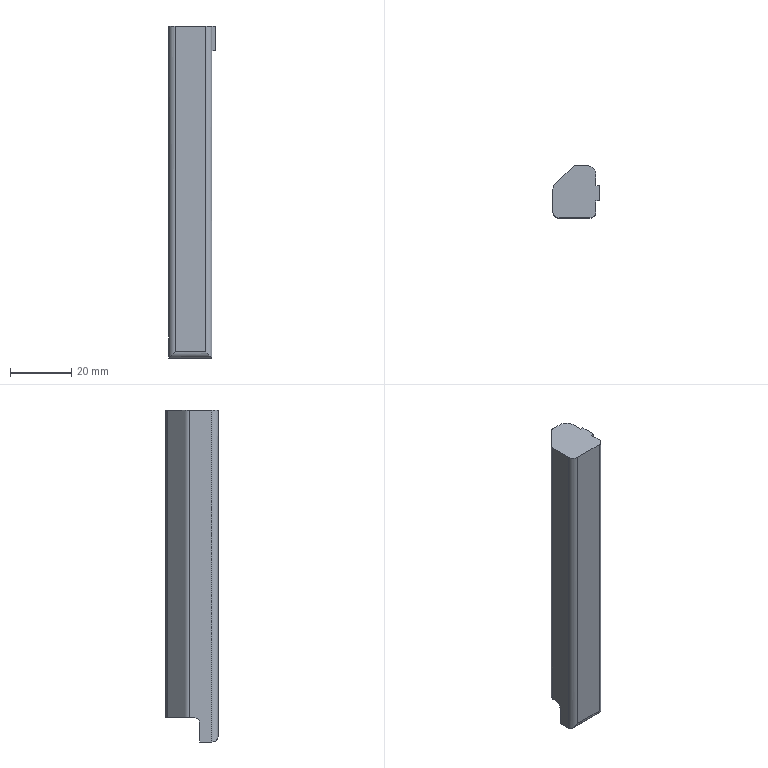Part | STEP file | PN_0026_id138_x_t | 1 solid | 20 faces | box 15 x 17 x 108 mm | volume 21787 mm3 | plane 13 | cylinder 5 | other 2 | commonest cylinder face diameters 4 x5
STEP:
#1=CARTESIAN_POINT('',(-194.5,-111.,95.));
#2=VERTEX_POINT('',#1);
#3=CARTESIAN_POINT('',(-194.5,-111.,-13.));
#4=VERTEX_POINT('',#3);
#5=CARTESIAN_POINT('',(-194.5,-111.,48.6));
#6=DIRECTION('',(0.,0.,-1.));
#7=VECTOR('',#6,1.);
#8=LINE('',#5,#7);
#9=EDGE_CURVE('',#2,#4,#8,.T.);
#10=ORIENTED_EDGE('',*,*,#9,.T.);
#11=CARTESIAN_POINT('',(-194.5,-107.,-13.));
#12=VERTEX_POINT('',#11);
#13=CARTESIAN_POINT('',(-194.5,-99.,-13.));
#14=DIRECTION('',(0.,-1.,0.));
#15=VECTOR('',#14,1.);
#16=LINE('',#13,#15);
#17=EDGE_CURVE('',#12,#4,#16,.T.);
#18=ORIENTED_EDGE('',*,*,#17,.F.);
#19=CARTESIAN_POINT('',(-194.5,-107.,-7.));
#20=VERTEX_POINT('',#19);
#21=CARTESIAN_POINT('',(-194.5,-107.,23.6));
#22=DIRECTION('',(0.,0.,1.));
#23=VECTOR('',#22,1.);
#24=LINE('',#21,#23);
#25=EDGE_CURVE('',#12,#20,#24,.T.);
#26=ORIENTED_EDGE('',*,*,#25,.T.);
#27=CARTESIAN_POINT('',(-194.5,-105.,-5.));
#28=VERTEX_POINT('',#27);
#29=CARTESIAN_POINT('',(-194.5,-105.,-7.));
#30=DIRECTION('',(-1.,0.,0.));
#31=DIRECTION('',(0.,0.,-1.));
#32=AXIS2_PLACEMENT_3D('',#29,#30,#31);
#33=CIRCLE('',#32,2.);
#34=EDGE_CURVE('',#20,#28,#33,.T.);
#35=ORIENTED_EDGE('',*,*,#34,.T.);
#36=CARTESIAN_POINT('',(-194.5,-99.,-5.));
#37=VERTEX_POINT('',#36);
#38=CARTESIAN_POINT('',(-194.5,-83.97,-5.));
#39=CARTESIAN_POINT('',(-194.5,-85.287,-5.));
#40=CARTESIAN_POINT('',(-194.5,-86.605,-5.));
#41=CARTESIAN_POINT('',(-194.5,-87.923,-5.));
#42=CARTESIAN_POINT('',(-194.5,-88.936,-5.));
#43=CARTESIAN_POINT('',(-194.5,-89.95,-5.));
#44=CARTESIAN_POINT('',(-194.5,-90.964,-5.));
#45=CARTESIAN_POINT('',(-194.5,-91.743,-5.));
#46=CARTESIAN_POINT('',(-194.5,-92.523,-5.));
#47=CARTESIAN_POINT('',(-194.5,-93.303,-5.));
#48=CARTESIAN_POINT('',(-194.5,-93.903,-5.));
#49=CARTESIAN_POINT('',(-194.5,-94.502,-5.));
#50=CARTESIAN_POINT('',(-194.5,-95.102,-5.));
#51=CARTESIAN_POINT('',(-194.5,-95.564,-5.));
#52=CARTESIAN_POINT('',(-194.5,-96.025,-5.));
#53=CARTESIAN_POINT('',(-194.5,-96.486,-5.));
#54=CARTESIAN_POINT('',(-194.5,-96.841,-5.));
#55=CARTESIAN_POINT('',(-194.5,-97.196,-5.));
#56=CARTESIAN_POINT('',(-194.5,-97.551,-5.));
#57=CARTESIAN_POINT('',(-194.5,-97.824,-5.));
#58=CARTESIAN_POINT('',(-194.5,-98.097,-5.));
#59=CARTESIAN_POINT('',(-194.5,-98.37,-5.));
#60=CARTESIAN_POINT('',(-194.5,-98.58,-5.));
#61=CARTESIAN_POINT('',(-194.5,-98.79,-5.));
#62=CARTESIAN_POINT('',(-194.5,-99.,-5.));
#63=CARTESIAN_POINT('',(-194.5,-99.667,-5.));
#64=CARTESIAN_POINT('',(-194.5,-100.333,-5.));
#65=CARTESIAN_POINT('',(-194.5,-101.,-5.));
#66=CARTESIAN_POINT('',(-194.5,-101.733,-5.));
#67=CARTESIAN_POINT('',(-194.5,-102.467,-5.));
#68=CARTESIAN_POINT('',(-194.5,-103.2,-5.));
#69=CARTESIAN_POINT('',(-194.5,-103.41,-5.));
#70=CARTESIAN_POINT('',(-194.5,-103.62,-5.));
#71=CARTESIAN_POINT('',(-194.5,-103.83,-5.));
#72=CARTESIAN_POINT('',(-194.5,-104.103,-5.));
#73=CARTESIAN_POINT('',(-194.5,-104.376,-5.));
#74=CARTESIAN_POINT('',(-194.5,-104.649,-5.));
#75=CARTESIAN_POINT('',(-194.5,-105.004,-5.));
#76=CARTESIAN_POINT('',(-194.5,-105.359,-5.));
#77=CARTESIAN_POINT('',(-194.5,-105.714,-5.));
#78=CARTESIAN_POINT('',(-194.5,-106.175,-5.));
#79=CARTESIAN_POINT('',(-194.5,-106.636,-5.));
#80=CARTESIAN_POINT('',(-194.5,-107.098,-5.));
#81=CARTESIAN_POINT('',(-194.5,-107.698,-5.));
#82=CARTESIAN_POINT('',(-194.5,-108.297,-5.));
#83=CARTESIAN_POINT('',(-194.5,-108.897,-5.));
#84=CARTESIAN_POINT('',(-194.5,-109.677,-5.));
#85=CARTESIAN_POINT('',(-194.5,-110.457,-5.));
#86=CARTESIAN_POINT('',(-194.5,-111.236,-5.));
#87=CARTESIAN_POINT('',(-194.5,-112.25,-5.));
#88=CARTESIAN_POINT('',(-194.5,-113.264,-5.));
#89=CARTESIAN_POINT('',(-194.5,-114.277,-5.));
#90=CARTESIAN_POINT('',(-194.5,-115.595,-5.));
#91=CARTESIAN_POINT('',(-194.5,-116.913,-5.));
#92=CARTESIAN_POINT('',(-194.5,-118.23,-5.));
#93=B_SPLINE_CURVE_WITH_KNOTS('',3,(#38,#39,#40,#41,#42,#43,#44,#45,#46,#47,#48,#49,#50,#51,#52,#53,#54,#55,#56,#57,#58,#59,#60,#61,#62,#63,#64,#65,#66,#67,#68,#69,#70,#71,#72,#73,#74,#75,#76,#77,#78,#79,#80,#81,#82,#83,#84,#85,#86,#87,#88,#89,#90,#91,#92),.UNSPECIFIED.,.F.,.F.,(4,3,3,3,3,3,3,3,3,3,3,3,3,3,3,3,3,3,4),(0.,0.1154,0.2041,0.2724,0.3249,0.3653,0.3964,0.4203,0.4387,0.4971,0.5613,0.5797,0.6036,0.6347,0.6751,0.7276,0.7959,0.8846,1.),.UNSPECIFIED.);
#94=EDGE_CURVE('',#37,#28,#93,.T.);
#95=ORIENTED_EDGE('',*,*,#94,.F.);
#96=CARTESIAN_POINT('',(-194.5,-99.,95.));
#97=VERTEX_POINT('',#96);
#98=CARTESIAN_POINT('',(-194.5,-99.,48.6));
#99=DIRECTION('',(0.,0.,-1.));
#100=VECTOR('',#99,1.);
#101=LINE('',#98,#100);
#102=EDGE_CURVE('',#97,#37,#101,.T.);
#103=ORIENTED_EDGE('',*,*,#102,.F.);
#104=CARTESIAN_POINT('',(-194.5,-102.5,95.));
#105=VERTEX_POINT('',#104);
#106=CARTESIAN_POINT('',(-194.5,-99.,95.));
#107=DIRECTION('',(0.,-1.,0.));
#108=VECTOR('',#107,1.);
#109=LINE('',#106,#108);
#110=EDGE_CURVE('',#97,#105,#109,.T.);
#111=ORIENTED_EDGE('',*,*,#110,.T.);
#112=CARTESIAN_POINT('',(-194.5,-102.5,87.));
#113=VERTEX_POINT('',#112);
#114=CARTESIAN_POINT('',(-194.5,-102.5,95.));
#115=DIRECTION('',(0.,0.,-1.));
#116=VECTOR('',#115,1.);
#117=LINE('',#114,#116);
#118=EDGE_CURVE('',#105,#113,#117,.T.);
#119=ORIENTED_EDGE('',*,*,#118,.T.);
#120=CARTESIAN_POINT('',(-194.5,-107.5,87.));
#121=VERTEX_POINT('',#120);
#122=CARTESIAN_POINT('',(-194.5,-102.5,87.));
#123=DIRECTION('',(0.,-1.,0.));
#124=VECTOR('',#123,1.);
#125=LINE('',#122,#124);
#126=EDGE_CURVE('',#113,#121,#125,.T.);
#127=ORIENTED_EDGE('',*,*,#126,.T.);
#128=CARTESIAN_POINT('',(-194.5,-107.5,95.));
#129=VERTEX_POINT('',#128);
#130=CARTESIAN_POINT('',(-194.5,-107.5,90.));
#131=DIRECTION('',(0.,0.,1.));
#132=VECTOR('',#131,1.);
#133=LINE('',#130,#132);
#134=EDGE_CURVE('',#121,#129,#133,.T.);
#135=ORIENTED_EDGE('',*,*,#134,.T.);
#136=CARTESIAN_POINT('',(-194.5,-99.,95.));
#137=DIRECTION('',(0.,-1.,0.));
#138=VECTOR('',#137,1.);
#139=LINE('',#136,#138);
#140=EDGE_CURVE('',#129,#2,#139,.T.);
#141=ORIENTED_EDGE('',*,*,#140,.T.);
#142=EDGE_LOOP('',(#10,#18,#26,#35,#95,#103,#111,#119,#127,#135,#141));
#143=FACE_OUTER_BOUND('',#142,.T.);
#144=CARTESIAN_POINT('',(-194.5,-99.,48.6));
#145=DIRECTION('',(1.,0.,0.));
#146=DIRECTION('',(0.,0.,-1.));
#147=AXIS2_PLACEMENT_3D('',#144,#145,#146);
#148=PLANE('',#147);
#149=ADVANCED_FACE('',(#143),#148,.T.);
#150=CARTESIAN_POINT('',(-206.5,-113.,95.));
#151=VERTEX_POINT('',#150);
#152=CARTESIAN_POINT('',(-206.5,-113.,-11.));
#153=VERTEX_POINT('',#152);
#154=CARTESIAN_POINT('',(-206.5,-113.,18.6));
#155=DIRECTION('',(0.,0.,-1.));
#156=VECTOR('',#155,1.);
#157=LINE('',#154,#156);
#158=EDGE_CURVE('',#151,#153,#157,.T.);
#159=ORIENTED_EDGE('',*,*,#158,.T.);
#160=CARTESIAN_POINT('',(-196.5,-113.,-11.));
#161=VERTEX_POINT('',#160);
#162=CARTESIAN_POINT('',(-196.5,-113.,-11.));
#163=DIRECTION('',(1.,0.,0.));
#164=VECTOR('',#163,1.);
#165=LINE('',#162,#164);
#166=EDGE_CURVE('',#153,#161,#165,.T.);
#167=ORIENTED_EDGE('',*,*,#166,.T.);
#168=CARTESIAN_POINT('',(-196.5,-113.,95.));
#169=VERTEX_POINT('',#168);
#170=CARTESIAN_POINT('',(-196.5,-113.,48.6));
#171=DIRECTION('',(0.,0.,1.));
#172=VECTOR('',#171,1.);
#173=LINE('',#170,#172);
#174=EDGE_CURVE('',#161,#169,#173,.T.);
#175=ORIENTED_EDGE('',*,*,#174,.T.);
#176=CARTESIAN_POINT('',(-194.5,-113.,95.));
#177=DIRECTION('',(-1.,0.,0.));
#178=VECTOR('',#177,1.);
#179=LINE('',#176,#178);
#180=EDGE_CURVE('',#169,#151,#179,.T.);
#181=ORIENTED_EDGE('',*,*,#180,.T.);
#182=EDGE_LOOP('',(#159,#167,#175,#181));
#183=FACE_OUTER_BOUND('',#182,.T.);
#184=CARTESIAN_POINT('',(-194.5,-113.,48.6));
#185=DIRECTION('',(0.,-1.,0.));
#186=DIRECTION('',(0.,0.,-1.));
#187=AXIS2_PLACEMENT_3D('',#184,#185,#186);
#188=PLANE('',#187);
#189=ADVANCED_FACE('',(#183),#188,.T.);
#190=ORIENTED_EDGE('',*,*,#174,.F.);
#191=CARTESIAN_POINT('',(-196.5,-111.,-11.));
#192=DIRECTION('',(0.7071,0.,0.7071));
#193=DIRECTION('',(0.7071,0.,-0.7071));
#194=AXIS2_PLACEMENT_3D('',#191,#192,#193);
#195=ELLIPSE('',#194,2.828,2.);
#196=EDGE_CURVE('',#161,#4,#195,.T.);
#197=ORIENTED_EDGE('',*,*,#196,.T.);
#198=ORIENTED_EDGE('',*,*,#9,.F.);
#199=CARTESIAN_POINT('',(-196.5,-111.,95.));
#200=DIRECTION('',(0.,0.,1.));
#201=DIRECTION('',(-1.,0.,0.));
#202=AXIS2_PLACEMENT_3D('',#199,#200,#201);
#203=CIRCLE('',#202,2.);
#204=EDGE_CURVE('',#169,#2,#203,.T.);
#205=ORIENTED_EDGE('',*,*,#204,.F.);
#206=EDGE_LOOP('',(#190,#197,#198,#205));
#207=FACE_OUTER_BOUND('',#206,.T.);
#208=CARTESIAN_POINT('',(-196.5,-111.,48.6));
#209=DIRECTION('',(0.,0.,-1.));
#210=DIRECTION('',(-1.,0.,0.));
#211=AXIS2_PLACEMENT_3D('',#208,#209,#210);
#212=CYLINDRICAL_SURFACE('',#211,2.);
#213=ADVANCED_FACE('',(#207),#212,.T.);
#214=CARTESIAN_POINT('',(-208.5,-111.,-13.));
#215=VERTEX_POINT('',#214);
#216=CARTESIAN_POINT('',(-208.5,-111.,95.));
#217=VERTEX_POINT('',#216);
#218=CARTESIAN_POINT('',(-208.5,-111.,48.6));
#219=DIRECTION('',(0.,0.,1.));
#220=VECTOR('',#219,1.);
#221=LINE('',#218,#220);
#222=EDGE_CURVE('',#215,#217,#221,.T.);
#223=ORIENTED_EDGE('',*,*,#222,.F.);
#224=CARTESIAN_POINT('',(-206.5,-111.,-11.));
#225=DIRECTION('',(-0.7071,0.,0.7071));
#226=DIRECTION('',(-0.7071,0.,-0.7071));
#227=AXIS2_PLACEMENT_3D('',#224,#225,#226);
#228=ELLIPSE('',#227,2.828,2.);
#229=EDGE_CURVE('',#215,#153,#228,.T.);
#230=ORIENTED_EDGE('',*,*,#229,.T.);
#231=ORIENTED_EDGE('',*,*,#158,.F.);
#232=CARTESIAN_POINT('',(-206.5,-111.,95.));
#233=DIRECTION('',(0.,0.,1.));
#234=DIRECTION('',(-1.,0.,0.));
#235=AXIS2_PLACEMENT_3D('',#232,#233,#234);
#236=CIRCLE('',#235,2.);
#237=EDGE_CURVE('',#217,#151,#236,.T.);
#238=ORIENTED_EDGE('',*,*,#237,.F.);
#239=EDGE_LOOP('',(#223,#230,#231,#238));
#240=FACE_OUTER_BOUND('',#239,.T.);
#241=CARTESIAN_POINT('',(-206.5,-111.,33.6));
#242=DIRECTION('',(0.,0.,-1.));
#243=DIRECTION('',(-1.,0.,0.));
#244=AXIS2_PLACEMENT_3D('',#241,#242,#243);
#245=CYLINDRICAL_SURFACE('',#244,2.);
#246=ADVANCED_FACE('',(#240),#245,.T.);
#247=CARTESIAN_POINT('',(-208.5,-103.657,95.));
#248=VERTEX_POINT('',#247);
#249=CARTESIAN_POINT('',(-208.5,-103.657,-5.));
#250=VERTEX_POINT('',#249);
#251=CARTESIAN_POINT('',(-208.5,-103.657,33.6));
#252=DIRECTION('',(0.,0.,-1.));
#253=VECTOR('',#252,1.);
#254=LINE('',#251,#253);
#255=EDGE_CURVE('',#248,#250,#254,.T.);
#256=ORIENTED_EDGE('',*,*,#255,.T.);
#257=CARTESIAN_POINT('',(-208.5,-105.,-5.));
#258=VERTEX_POINT('',#257);
#259=CARTESIAN_POINT('',(-208.5,-104.5,-5.));
#260=DIRECTION('',(0.,-1.,0.));
#261=VECTOR('',#260,1.);
#262=LINE('',#259,#261);
#263=EDGE_CURVE('',#250,#258,#262,.T.);
#264=ORIENTED_EDGE('',*,*,#263,.T.);
#265=CARTESIAN_POINT('',(-208.5,-107.,-7.));
#266=VERTEX_POINT('',#265);
#267=CARTESIAN_POINT('',(-208.5,-105.,-7.));
#268=DIRECTION('',(1.,0.,0.));
#269=DIRECTION('',(0.,0.,-1.));
#270=AXIS2_PLACEMENT_3D('',#267,#268,#269);
#271=CIRCLE('',#270,2.);
#272=EDGE_CURVE('',#258,#266,#271,.T.);
#273=ORIENTED_EDGE('',*,*,#272,.T.);
#274=CARTESIAN_POINT('',(-208.5,-107.,-13.));
#275=VERTEX_POINT('',#274);
#276=CARTESIAN_POINT('',(-208.5,-107.,8.6));
#277=DIRECTION('',(0.,0.,1.));
#278=VECTOR('',#277,1.);
#279=LINE('',#276,#278);
#280=EDGE_CURVE('',#275,#266,#279,.T.);
#281=ORIENTED_EDGE('',*,*,#280,.F.);
#282=CARTESIAN_POINT('',(-208.5,-104.5,-13.));
#283=DIRECTION('',(0.,-1.,0.));
#284=VECTOR('',#283,1.);
#285=LINE('',#282,#284);
#286=EDGE_CURVE('',#275,#215,#285,.T.);
#287=ORIENTED_EDGE('',*,*,#286,.T.);
#288=ORIENTED_EDGE('',*,*,#222,.T.);
#289=CARTESIAN_POINT('',(-208.5,-104.5,95.));
#290=DIRECTION('',(0.,-1.,0.));
#291=VECTOR('',#290,1.);
#292=LINE('',#289,#291);
#293=EDGE_CURVE('',#248,#217,#292,.T.);
#294=ORIENTED_EDGE('',*,*,#293,.F.);
#295=EDGE_LOOP('',(#256,#264,#273,#281,#287,#288,#294));
#296=FACE_OUTER_BOUND('',#295,.T.);
#297=CARTESIAN_POINT('',(-208.5,-104.5,33.6));
#298=DIRECTION('',(1.,0.,0.));
#299=DIRECTION('',(0.,0.,-1.));
#300=AXIS2_PLACEMENT_3D('',#297,#298,#299);
#301=PLANE('',#300);
#302=ADVANCED_FACE('',(#296),#301,.F.);
#303=ORIENTED_EDGE('',*,*,#110,.F.);
#304=CARTESIAN_POINT('',(-197.5,-96.,95.));
#305=VERTEX_POINT('',#304);
#306=CARTESIAN_POINT('',(-197.5,-96.,95.));
#307=CARTESIAN_POINT('',(-197.163,-96.,95.));
#308=CARTESIAN_POINT('',(-196.822,-96.058,95.));
#309=CARTESIAN_POINT('',(-196.504,-96.17,95.));
#310=CARTESIAN_POINT('',(-196.187,-96.282,95.));
#311=CARTESIAN_POINT('',(-195.883,-96.449,95.));
#312=CARTESIAN_POINT('',(-195.621,-96.661,95.));
#313=CARTESIAN_POINT('',(-195.36,-96.871,95.));
#314=CARTESIAN_POINT('',(-195.131,-97.128,95.));
#315=CARTESIAN_POINT('',(-194.954,-97.412,95.));
#316=CARTESIAN_POINT('',(-194.776,-97.698,95.));
#317=CARTESIAN_POINT('',(-194.645,-98.018,95.));
#318=CARTESIAN_POINT('',(-194.571,-98.347,95.));
#319=CARTESIAN_POINT('',(-194.524,-98.56,95.));
#320=CARTESIAN_POINT('',(-194.5,-98.781,95.));
#321=CARTESIAN_POINT('',(-194.5,-99.,95.));
#322=B_SPLINE_CURVE_WITH_KNOTS('',3,(#306,#307,#308,#309,#310,#311,#312,#313,#314,#315,#316,#317,#318,#319,#320,#321),.UNSPECIFIED.,.F.,.F.,(4,3,3,3,3,4),(0.,0.2157,0.4313,0.6456,0.861,1.),.UNSPECIFIED.);
#323=EDGE_CURVE('',#305,#97,#322,.T.);
#324=ORIENTED_EDGE('',*,*,#323,.F.);
#325=CARTESIAN_POINT('',(-200.843,-96.,95.));
#326=VERTEX_POINT('',#325);
#327=CARTESIAN_POINT('',(-200.843,-96.,95.));
#328=DIRECTION('',(1.,0.,0.));
#329=VECTOR('',#328,1.);
#330=LINE('',#327,#329);
#331=EDGE_CURVE('',#326,#305,#330,.T.);
#332=ORIENTED_EDGE('',*,*,#331,.F.);
#333=CARTESIAN_POINT('',(-202.257,-96.586,95.));
#334=VERTEX_POINT('',#333);
#335=CARTESIAN_POINT('',(-202.257,-96.586,95.));
#336=CARTESIAN_POINT('',(-202.164,-96.493,95.));
#337=CARTESIAN_POINT('',(-202.062,-96.408,95.));
#338=CARTESIAN_POINT('',(-201.952,-96.335,95.));
#339=CARTESIAN_POINT('',(-201.766,-96.211,95.));
#340=CARTESIAN_POINT('',(-201.555,-96.118,95.));
#341=CARTESIAN_POINT('',(-201.338,-96.062,95.));
#342=CARTESIAN_POINT('',(-201.177,-96.021,95.));
#343=CARTESIAN_POINT('',(-201.009,-96.,95.));
#344=CARTESIAN_POINT('',(-200.843,-96.,95.));
#345=B_SPLINE_CURVE_WITH_KNOTS('',3,(#335,#336,#337,#338,#339,#340,#341,#342,#343,#344),.UNSPECIFIED.,.F.,.F.,(4,3,3,4),(0.,0.2511,0.6821,1.),.UNSPECIFIED.);
#346=EDGE_CURVE('',#334,#326,#345,.T.);
#347=ORIENTED_EDGE('',*,*,#346,.F.);
#348=CARTESIAN_POINT('',(-207.914,-102.243,95.));
#349=VERTEX_POINT('',#348);
#350=CARTESIAN_POINT('',(-206.672,-101.,95.));
#351=DIRECTION('',(0.7071,0.7071,0.));
#352=VECTOR('',#351,1.);
#353=LINE('',#350,#352);
#354=EDGE_CURVE('',#349,#334,#353,.T.);
#355=ORIENTED_EDGE('',*,*,#354,.F.);
#356=CARTESIAN_POINT('',(-206.5,-103.657,95.));
#357=DIRECTION('',(0.,0.,1.));
#358=DIRECTION('',(-1.,0.,0.));
#359=AXIS2_PLACEMENT_3D('',#356,#357,#358);
#360=CIRCLE('',#359,2.);
#361=EDGE_CURVE('',#349,#248,#360,.T.);
#362=ORIENTED_EDGE('',*,*,#361,.T.);
#363=ORIENTED_EDGE('',*,*,#293,.T.);
#364=ORIENTED_EDGE('',*,*,#237,.T.);
#365=ORIENTED_EDGE('',*,*,#180,.F.);
#366=ORIENTED_EDGE('',*,*,#204,.T.);
#367=ORIENTED_EDGE('',*,*,#140,.F.);
#368=CARTESIAN_POINT('',(-193.5,-107.5,95.));
#369=VERTEX_POINT('',#368);
#370=CARTESIAN_POINT('',(-193.5,-107.5,95.));
#371=DIRECTION('',(-1.,0.,0.));
#372=VECTOR('',#371,1.);
#373=LINE('',#370,#372);
#374=EDGE_CURVE('',#369,#129,#373,.T.);
#375=ORIENTED_EDGE('',*,*,#374,.F.);
#376=CARTESIAN_POINT('',(-193.5,-102.5,95.));
#377=VERTEX_POINT('',#376);
#378=CARTESIAN_POINT('',(-193.5,-107.5,95.));
#379=DIRECTION('',(0.,1.,0.));
#380=VECTOR('',#379,1.);
#381=LINE('',#378,#380);
#382=EDGE_CURVE('',#369,#377,#381,.T.);
#383=ORIENTED_EDGE('',*,*,#382,.T.);
#384=CARTESIAN_POINT('',(-193.5,-102.5,95.));
#385=DIRECTION('',(-1.,0.,0.));
#386=VECTOR('',#385,1.);
#387=LINE('',#384,#386);
#388=EDGE_CURVE('',#377,#105,#387,.T.);
#389=ORIENTED_EDGE('',*,*,#388,.T.);
#390=EDGE_LOOP('',(#303,#324,#332,#347,#355,#362,#363,#364,#365,#366,#367,#375,#383,#389));
#391=FACE_OUTER_BOUND('',#390,.T.);
#392=CARTESIAN_POINT('',(-114.973,24.687,95.));
#393=DIRECTION('',(0.,0.,-1.));
#394=DIRECTION('',(-1.,0.,0.));
#395=AXIS2_PLACEMENT_3D('',#392,#393,#394);
#396=PLANE('',#395);
#397=ADVANCED_FACE('',(#391),#396,.F.);
#398=CARTESIAN_POINT('',(-202.257,-96.586,-5.));
#399=VERTEX_POINT('',#398);
#400=CARTESIAN_POINT('',(-202.257,-96.586,48.6));
#401=DIRECTION('',(0.,0.,-1.));
#402=VECTOR('',#401,1.);
#403=LINE('',#400,#402);
#404=EDGE_CURVE('',#334,#399,#403,.T.);
#405=ORIENTED_EDGE('',*,*,#404,.T.);
#406=CARTESIAN_POINT('',(-207.914,-102.243,-5.));
#407=VERTEX_POINT('',#406);
#408=CARTESIAN_POINT('',(-218.322,-112.651,-5.));
#409=CARTESIAN_POINT('',(-217.299,-111.627,-5.));
#410=CARTESIAN_POINT('',(-216.275,-110.604,-5.));
#411=CARTESIAN_POINT('',(-215.251,-109.58,-5.));
#412=CARTESIAN_POINT('',(-214.464,-108.792,-5.));
#413=CARTESIAN_POINT('',(-213.676,-108.005,-5.));
#414=CARTESIAN_POINT('',(-212.889,-107.217,-5.));
#415=CARTESIAN_POINT('',(-212.283,-106.612,-5.));
#416=CARTESIAN_POINT('',(-211.678,-106.006,-5.));
#417=CARTESIAN_POINT('',(-211.072,-105.4,-5.));
#418=CARTESIAN_POINT('',(-210.606,-104.934,-5.));
#419=CARTESIAN_POINT('',(-210.14,-104.468,-5.));
#420=CARTESIAN_POINT('',(-209.674,-104.002,-5.));
#421=CARTESIAN_POINT('',(-209.316,-103.644,-5.));
#422=CARTESIAN_POINT('',(-208.957,-103.286,-5.));
#423=CARTESIAN_POINT('',(-208.599,-102.927,-5.));
#424=CARTESIAN_POINT('',(-208.323,-102.651,-5.));
#425=CARTESIAN_POINT('',(-208.047,-102.376,-5.));
#426=CARTESIAN_POINT('',(-207.772,-102.1,-5.));
#427=CARTESIAN_POINT('',(-207.405,-101.733,-5.));
#428=CARTESIAN_POINT('',(-207.038,-101.367,-5.));
#429=CARTESIAN_POINT('',(-206.672,-101.,-5.));
#430=CARTESIAN_POINT('',(-205.2,-99.529,-5.));
#431=CARTESIAN_POINT('',(-203.729,-98.057,-5.));
#432=CARTESIAN_POINT('',(-202.257,-96.586,-5.));
#433=CARTESIAN_POINT('',(-201.982,-96.31,-5.));
#434=CARTESIAN_POINT('',(-201.706,-96.034,-5.));
#435=CARTESIAN_POINT('',(-201.43,-95.759,-5.));
#436=CARTESIAN_POINT('',(-201.072,-95.4,-5.));
#437=CARTESIAN_POINT('',(-200.713,-95.042,-5.));
#438=CARTESIAN_POINT('',(-200.355,-94.683,-5.));
#439=CARTESIAN_POINT('',(-199.889,-94.217,-5.));
#440=CARTESIAN_POINT('',(-199.423,-93.751,-5.));
#441=CARTESIAN_POINT('',(-198.957,-93.286,-5.));
#442=CARTESIAN_POINT('',(-198.351,-92.68,-5.));
#443=CARTESIAN_POINT('',(-197.746,-92.074,-5.));
#444=CARTESIAN_POINT('',(-197.14,-91.468,-5.));
#445=CARTESIAN_POINT('',(-196.352,-90.681,-5.));
#446=CARTESIAN_POINT('',(-195.565,-89.893,-5.));
#447=CARTESIAN_POINT('',(-194.778,-89.106,-5.));
#448=CARTESIAN_POINT('',(-193.754,-88.082,-5.));
#449=CARTESIAN_POINT('',(-192.73,-87.059,-5.));
#450=CARTESIAN_POINT('',(-191.706,-86.035,-5.));
#451=B_SPLINE_CURVE_WITH_KNOTS('',3,(#408,#409,#410,#411,#412,#413,#414,#415,#416,#417,#418,#419,#420,#421,#422,#423,#424,#425,#426,#427,#428,#429,#430,#431,#432,#433,#434,#435,#436,#437,#438,#439,#440,#441,#442,#443,#444,#445,#446,#447,#448,#449,#450),.UNSPECIFIED.,.F.,.F.,(4,3,3,3,3,3,3,3,3,3,3,3,3,3,4),(0.,0.1154,0.2041,0.2724,0.3249,0.3653,0.3964,0.4377,0.6036,0.6347,0.6751,0.7276,0.7959,0.8846,1.),.UNSPECIFIED.);
#452=EDGE_CURVE('',#407,#399,#451,.T.);
#453=ORIENTED_EDGE('',*,*,#452,.F.);
#454=CARTESIAN_POINT('',(-207.914,-102.243,48.6));
#455=DIRECTION('',(0.,0.,1.));
#456=VECTOR('',#455,1.);
#457=LINE('',#454,#456);
#458=EDGE_CURVE('',#407,#349,#457,.T.);
#459=ORIENTED_EDGE('',*,*,#458,.T.);
#460=ORIENTED_EDGE('',*,*,#354,.T.);
#461=EDGE_LOOP('',(#405,#453,#459,#460));
#462=FACE_OUTER_BOUND('',#461,.T.);
#463=CARTESIAN_POINT('',(-206.672,-101.,48.6));
#464=DIRECTION('',(-0.7071,0.7071,0.));
#465=DIRECTION('',(-0.7071,-0.7071,0.));
#466=AXIS2_PLACEMENT_3D('',#463,#464,#465);
#467=PLANE('',#466);
#468=ADVANCED_FACE('',(#462),#467,.T.);
#469=CARTESIAN_POINT('',(-200.843,-96.,-5.));
#470=VERTEX_POINT('',#469);
#471=CARTESIAN_POINT('',(-200.843,-96.,48.6));
#472=DIRECTION('',(0.,0.,-1.));
#473=VECTOR('',#472,1.);
#474=LINE('',#471,#473);
#475=EDGE_CURVE('',#326,#470,#474,.T.);
#476=ORIENTED_EDGE('',*,*,#475,.T.);
#477=CARTESIAN_POINT('',(-202.257,-96.586,-5.));
#478=CARTESIAN_POINT('',(-202.211,-96.54,-5.));
#479=CARTESIAN_POINT('',(-202.114,-96.451,-5.));
#480=CARTESIAN_POINT('',(-201.956,-96.334,-5.));
#481=CARTESIAN_POINT('',(-201.788,-96.233,-5.));
#482=CARTESIAN_POINT('',(-201.61,-96.149,-5.));
#483=CARTESIAN_POINT('',(-201.425,-96.083,-5.));
#484=CARTESIAN_POINT('',(-201.234,-96.035,-5.));
#485=CARTESIAN_POINT('',(-201.04,-96.006,-5.));
#486=CARTESIAN_POINT('',(-200.909,-96.,-5.));
#487=CARTESIAN_POINT('',(-200.843,-96.,-5.));
#488=B_SPLINE_CURVE_WITH_KNOTS('',3,(#477,#478,#479,#480,#481,#482,#483,#484,#485,#486,#487),.UNSPECIFIED.,.F.,.F.,(4,1,1,1,1,1,1,1,4),(0.,0.125,0.25,0.375,0.5,0.625,0.75,0.875,1.),.UNSPECIFIED.);
#489=EDGE_CURVE('',#399,#470,#488,.T.);
#490=ORIENTED_EDGE('',*,*,#489,.F.);
#491=ORIENTED_EDGE('',*,*,#404,.F.);
#492=ORIENTED_EDGE('',*,*,#346,.T.);
#493=EDGE_LOOP('',(#476,#490,#491,#492));
#494=FACE_OUTER_BOUND('',#493,.T.);
#495=CARTESIAN_POINT('',(-202.257,-96.586,48.6));
#496=CARTESIAN_POINT('',(-202.211,-96.54,48.6));
#497=CARTESIAN_POINT('',(-202.114,-96.451,48.6));
#498=CARTESIAN_POINT('',(-201.956,-96.334,48.6));
#499=CARTESIAN_POINT('',(-201.788,-96.233,48.6));
#500=CARTESIAN_POINT('',(-201.61,-96.149,48.6));
#501=CARTESIAN_POINT('',(-201.425,-96.083,48.6));
#502=CARTESIAN_POINT('',(-201.234,-96.035,48.6));
#503=CARTESIAN_POINT('',(-201.04,-96.006,48.6));
#504=CARTESIAN_POINT('',(-200.909,-96.,48.6));
#505=CARTESIAN_POINT('',(-200.843,-96.,48.6));
#506=B_SPLINE_CURVE_WITH_KNOTS('',3,(#495,#496,#497,#498,#499,#500,#501,#502,#503,#504,#505),.UNSPECIFIED.,.F.,.F.,(4,1,1,1,1,1,1,1,4),(0.,0.125,0.25,0.375,0.5,0.625,0.75,0.875,1.),.UNSPECIFIED.);
#507=DIRECTION('',(0.,0.,-1.));
#508=VECTOR('',#507,1.);
#509=SURFACE_OF_LINEAR_EXTRUSION('',#506,#508);
#510=ADVANCED_FACE('',(#494),#509,.T.);
#511=CARTESIAN_POINT('',(-197.5,-96.,-5.));
#512=VERTEX_POINT('',#511);
#513=CARTESIAN_POINT('',(-197.5,-96.,48.6));
#514=DIRECTION('',(0.,0.,-1.));
#515=VECTOR('',#514,1.);
#516=LINE('',#513,#515);
#517=EDGE_CURVE('',#305,#512,#516,.T.);
#518=ORIENTED_EDGE('',*,*,#517,.T.);
#519=CARTESIAN_POINT('',(-200.843,-96.,-5.));
#520=CARTESIAN_POINT('',(-199.729,-96.,-5.));
#521=CARTESIAN_POINT('',(-198.614,-96.,-5.));
#522=CARTESIAN_POINT('',(-197.5,-96.,-5.));
#523=B_SPLINE_CURVE_WITH_KNOTS('',3,(#519,#520,#521,#522),.UNSPECIFIED.,.F.,.F.,(4,4),(0.,1.),.UNSPECIFIED.);
#524=EDGE_CURVE('',#470,#512,#523,.T.);
#525=ORIENTED_EDGE('',*,*,#524,.F.);
#526=ORIENTED_EDGE('',*,*,#475,.F.);
#527=ORIENTED_EDGE('',*,*,#331,.T.);
#528=EDGE_LOOP('',(#518,#525,#526,#527));
#529=FACE_OUTER_BOUND('',#528,.T.);
#530=CARTESIAN_POINT('',(-200.843,-96.,48.6));
#531=DIRECTION('',(0.,1.,0.));
#532=DIRECTION('',(0.,0.,1.));
#533=AXIS2_PLACEMENT_3D('',#530,#531,#532);
#534=PLANE('',#533);
#535=ADVANCED_FACE('',(#529),#534,.T.);
#536=ORIENTED_EDGE('',*,*,#102,.T.);
#537=CARTESIAN_POINT('',(-197.5,-96.,-5.));
#538=CARTESIAN_POINT('',(-197.402,-96.,-5.));
#539=CARTESIAN_POINT('',(-197.205,-96.009,-5.));
#540=CARTESIAN_POINT('',(-196.816,-96.067,-5.));
#541=CARTESIAN_POINT('',(-196.345,-96.211,-5.));
#542=CARTESIAN_POINT('',(-195.822,-96.488,-5.));
#543=CARTESIAN_POINT('',(-195.365,-96.865,-5.));
#544=CARTESIAN_POINT('',(-194.988,-97.322,-5.));
#545=CARTESIAN_POINT('',(-194.711,-97.845,-5.));
#546=CARTESIAN_POINT('',(-194.567,-98.316,-5.));
#547=CARTESIAN_POINT('',(-194.509,-98.705,-5.));
#548=CARTESIAN_POINT('',(-194.5,-98.902,-5.));
#549=CARTESIAN_POINT('',(-194.5,-99.,-5.));
#550=B_SPLINE_CURVE_WITH_KNOTS('',3,(#537,#538,#539,#540,#541,#542,#543,#544,#545,#546,#547,#548,#549),.UNSPECIFIED.,.F.,.F.,(4,1,1,1,1,1,1,1,1,1,4),(0.,0.0625,0.125,0.25,0.375,0.5,0.625,0.75,0.875,0.9375,1.),.UNSPECIFIED.);
#551=EDGE_CURVE('',#512,#37,#550,.T.);
#552=ORIENTED_EDGE('',*,*,#551,.F.);
#553=ORIENTED_EDGE('',*,*,#517,.F.);
#554=ORIENTED_EDGE('',*,*,#323,.T.);
#555=EDGE_LOOP('',(#536,#552,#553,#554));
#556=FACE_OUTER_BOUND('',#555,.T.);
#557=CARTESIAN_POINT('',(-197.5,-96.,48.6));
#558=CARTESIAN_POINT('',(-197.402,-96.,48.6));
#559=CARTESIAN_POINT('',(-197.205,-96.009,48.6));
#560=CARTESIAN_POINT('',(-196.816,-96.067,48.6));
#561=CARTESIAN_POINT('',(-196.345,-96.211,48.6));
#562=CARTESIAN_POINT('',(-195.822,-96.488,48.6));
#563=CARTESIAN_POINT('',(-195.365,-96.865,48.6));
#564=CARTESIAN_POINT('',(-194.988,-97.322,48.6));
#565=CARTESIAN_POINT('',(-194.711,-97.845,48.6));
#566=CARTESIAN_POINT('',(-194.567,-98.316,48.6));
#567=CARTESIAN_POINT('',(-194.509,-98.705,48.6));
#568=CARTESIAN_POINT('',(-194.5,-98.902,48.6));
#569=CARTESIAN_POINT('',(-194.5,-99.,48.6));
#570=B_SPLINE_CURVE_WITH_KNOTS('',3,(#557,#558,#559,#560,#561,#562,#563,#564,#565,#566,#567,#568,#569),.UNSPECIFIED.,.F.,.F.,(4,1,1,1,1,1,1,1,1,1,4),(0.,0.0625,0.125,0.25,0.375,0.5,0.625,0.75,0.875,0.9375,1.),.UNSPECIFIED.);
#571=DIRECTION('',(0.,0.,-1.));
#572=VECTOR('',#571,1.);
#573=SURFACE_OF_LINEAR_EXTRUSION('',#570,#572);
#574=ADVANCED_FACE('',(#556),#573,.T.);
#575=ORIENTED_EDGE('',*,*,#458,.F.);
#576=CARTESIAN_POINT('',(-206.5,-103.657,-5.));
#577=DIRECTION('',(0.,0.,-1.));
#578=DIRECTION('',(1.,0.,0.));
#579=AXIS2_PLACEMENT_3D('',#576,#577,#578);
#580=CIRCLE('',#579,2.);
#581=EDGE_CURVE('',#250,#407,#580,.T.);
#582=ORIENTED_EDGE('',*,*,#581,.F.);
#583=ORIENTED_EDGE('',*,*,#255,.F.);
#584=ORIENTED_EDGE('',*,*,#361,.F.);
#585=EDGE_LOOP('',(#575,#582,#583,#584));
#586=FACE_OUTER_BOUND('',#585,.T.);
#587=CARTESIAN_POINT('',(-206.5,-103.657,33.6));
#588=DIRECTION('',(0.,0.,1.));
#589=DIRECTION('',(1.,0.,0.));
#590=AXIS2_PLACEMENT_3D('',#587,#588,#589);
#591=CYLINDRICAL_SURFACE('',#590,2.);
#592=ADVANCED_FACE('',(#586),#591,.T.);
#593=ORIENTED_EDGE('',*,*,#126,.F.);
#594=CARTESIAN_POINT('',(-193.5,-102.5,87.));
#595=VERTEX_POINT('',#594);
#596=CARTESIAN_POINT('',(-193.5,-102.5,87.));
#597=DIRECTION('',(-1.,0.,0.));
#598=VECTOR('',#597,1.);
#599=LINE('',#596,#598);
#600=EDGE_CURVE('',#595,#113,#599,.T.);
#601=ORIENTED_EDGE('',*,*,#600,.F.);
#602=CARTESIAN_POINT('',(-193.5,-107.5,87.));
#603=VERTEX_POINT('',#602);
#604=CARTESIAN_POINT('',(-193.5,14.,87.));
#605=DIRECTION('',(0.,-1.,0.));
#606=VECTOR('',#605,1.);
#607=LINE('',#604,#606);
#608=EDGE_CURVE('',#595,#603,#607,.T.);
#609=ORIENTED_EDGE('',*,*,#608,.T.);
#610=CARTESIAN_POINT('',(-193.5,-107.5,87.));
#611=DIRECTION('',(-1.,0.,0.));
#612=VECTOR('',#611,1.);
#613=LINE('',#610,#612);
#614=EDGE_CURVE('',#603,#121,#613,.T.);
#615=ORIENTED_EDGE('',*,*,#614,.T.);
#616=EDGE_LOOP('',(#593,#601,#609,#615));
#617=FACE_OUTER_BOUND('',#616,.T.);
#618=CARTESIAN_POINT('',(-193.5,-102.5,87.));
#619=DIRECTION('',(0.,0.,-1.));
#620=DIRECTION('',(-1.,0.,0.));
#621=AXIS2_PLACEMENT_3D('',#618,#619,#620);
#622=PLANE('',#621);
#623=ADVANCED_FACE('',(#617),#622,.T.);
#624=ORIENTED_EDGE('',*,*,#134,.F.);
#625=ORIENTED_EDGE('',*,*,#614,.F.);
#626=CARTESIAN_POINT('',(-193.5,-107.5,90.));
#627=DIRECTION('',(0.,0.,1.));
#628=VECTOR('',#627,1.);
#629=LINE('',#626,#628);
#630=EDGE_CURVE('',#603,#369,#629,.T.);
#631=ORIENTED_EDGE('',*,*,#630,.T.);
#632=ORIENTED_EDGE('',*,*,#374,.T.);
#633=EDGE_LOOP('',(#624,#625,#631,#632));
#634=FACE_OUTER_BOUND('',#633,.T.);
#635=CARTESIAN_POINT('',(-193.5,-107.5,90.));
#636=DIRECTION('',(0.,-1.,0.));
#637=DIRECTION('',(0.,0.,-1.));
#638=AXIS2_PLACEMENT_3D('',#635,#636,#637);
#639=PLANE('',#638);
#640=ADVANCED_FACE('',(#634),#639,.T.);
#641=ORIENTED_EDGE('',*,*,#118,.F.);
#642=ORIENTED_EDGE('',*,*,#388,.F.);
#643=CARTESIAN_POINT('',(-193.5,-102.5,95.));
#644=DIRECTION('',(0.,0.,-1.));
#645=VECTOR('',#644,1.);
#646=LINE('',#643,#645);
#647=EDGE_CURVE('',#377,#595,#646,.T.);
#648=ORIENTED_EDGE('',*,*,#647,.T.);
#649=ORIENTED_EDGE('',*,*,#600,.T.);
#650=EDGE_LOOP('',(#641,#642,#648,#649));
#651=FACE_OUTER_BOUND('',#650,.T.);
#652=CARTESIAN_POINT('',(-193.5,-102.5,95.));
#653=DIRECTION('',(0.,1.,0.));
#654=DIRECTION('',(0.,0.,1.));
#655=AXIS2_PLACEMENT_3D('',#652,#653,#654);
#656=PLANE('',#655);
#657=ADVANCED_FACE('',(#651),#656,.T.);
#658=ORIENTED_EDGE('',*,*,#608,.F.);
#659=ORIENTED_EDGE('',*,*,#647,.F.);
#660=ORIENTED_EDGE('',*,*,#382,.F.);
#661=ORIENTED_EDGE('',*,*,#630,.F.);
#662=EDGE_LOOP('',(#658,#659,#660,#661));
#663=FACE_OUTER_BOUND('',#662,.T.);
#664=CARTESIAN_POINT('',(-193.5,14.,18.6));
#665=DIRECTION('',(-1.,0.,0.));
#666=DIRECTION('',(0.,0.,1.));
#667=AXIS2_PLACEMENT_3D('',#664,#665,#666);
#668=PLANE('',#667);
#669=ADVANCED_FACE('',(#663),#668,.F.);
#670=ORIENTED_EDGE('',*,*,#196,.F.);
#671=ORIENTED_EDGE('',*,*,#166,.F.);
#672=ORIENTED_EDGE('',*,*,#229,.F.);
#673=CARTESIAN_POINT('',(-206.5,-111.,-13.));
#674=DIRECTION('',(-1.,0.,0.));
#675=VECTOR('',#674,1.);
#676=LINE('',#673,#675);
#677=EDGE_CURVE('',#4,#215,#676,.T.);
#678=ORIENTED_EDGE('',*,*,#677,.F.);
#679=EDGE_LOOP('',(#670,#671,#672,#678));
#680=FACE_OUTER_BOUND('',#679,.T.);
#681=CARTESIAN_POINT('',(-201.609,-111.,-11.));
#682=DIRECTION('',(1.,0.,0.));
#683=DIRECTION('',(0.,0.,-1.));
#684=AXIS2_PLACEMENT_3D('',#681,#682,#683);
#685=CYLINDRICAL_SURFACE('',#684,2.);
#686=ADVANCED_FACE('',(#680),#685,.T.);
#687=ORIENTED_EDGE('',*,*,#17,.T.);
#688=ORIENTED_EDGE('',*,*,#677,.T.);
#689=ORIENTED_EDGE('',*,*,#286,.F.);
#690=CARTESIAN_POINT('',(-201.609,-107.,-13.));
#691=DIRECTION('',(1.,0.,0.));
#692=VECTOR('',#691,1.);
#693=LINE('',#690,#692);
#694=EDGE_CURVE('',#275,#12,#693,.T.);
#695=ORIENTED_EDGE('',*,*,#694,.T.);
#696=EDGE_LOOP('',(#687,#688,#689,#695));
#697=FACE_OUTER_BOUND('',#696,.T.);
#698=CARTESIAN_POINT('',(-201.609,-96.152,-13.));
#699=DIRECTION('',(0.,0.,1.));
#700=DIRECTION('',(1.,0.,0.));
#701=AXIS2_PLACEMENT_3D('',#698,#699,#700);
#702=PLANE('',#701);
#703=ADVANCED_FACE('',(#697),#702,.F.);
#704=ORIENTED_EDGE('',*,*,#280,.T.);
#705=CARTESIAN_POINT('',(-194.5,-107.,-7.));
#706=DIRECTION('',(1.,0.,0.));
#707=VECTOR('',#706,1.);
#708=LINE('',#705,#707);
#709=EDGE_CURVE('',#266,#20,#708,.T.);
#710=ORIENTED_EDGE('',*,*,#709,.T.);
#711=ORIENTED_EDGE('',*,*,#25,.F.);
#712=ORIENTED_EDGE('',*,*,#694,.F.);
#713=EDGE_LOOP('',(#704,#710,#711,#712));
#714=FACE_OUTER_BOUND('',#713,.T.);
#715=CARTESIAN_POINT('',(-201.5,-107.,23.6));
#716=DIRECTION('',(0.,-1.,0.));
#717=DIRECTION('',(0.,0.,-1.));
#718=AXIS2_PLACEMENT_3D('',#715,#716,#717);
#719=PLANE('',#718);
#720=ADVANCED_FACE('',(#714),#719,.F.);
#721=ORIENTED_EDGE('',*,*,#34,.F.);
#722=ORIENTED_EDGE('',*,*,#709,.F.);
#723=ORIENTED_EDGE('',*,*,#272,.F.);
#724=CARTESIAN_POINT('',(-208.5,-105.,-5.));
#725=DIRECTION('',(-1.,0.,0.));
#726=VECTOR('',#725,1.);
#727=LINE('',#724,#726);
#728=EDGE_CURVE('',#28,#258,#727,.T.);
#729=ORIENTED_EDGE('',*,*,#728,.F.);
#730=EDGE_LOOP('',(#721,#722,#723,#729));
#731=FACE_OUTER_BOUND('',#730,.T.);
#732=CARTESIAN_POINT('',(-201.609,-105.,-7.));
#733=DIRECTION('',(1.,0.,0.));
#734=DIRECTION('',(0.,0.,-1.));
#735=AXIS2_PLACEMENT_3D('',#732,#733,#734);
#736=CYLINDRICAL_SURFACE('',#735,2.);
#737=ADVANCED_FACE('',(#731),#736,.F.);
#738=ORIENTED_EDGE('',*,*,#94,.T.);
#739=ORIENTED_EDGE('',*,*,#728,.T.);
#740=ORIENTED_EDGE('',*,*,#263,.F.);
#741=ORIENTED_EDGE('',*,*,#581,.T.);
#742=ORIENTED_EDGE('',*,*,#452,.T.);
#743=ORIENTED_EDGE('',*,*,#489,.T.);
#744=ORIENTED_EDGE('',*,*,#524,.T.);
#745=ORIENTED_EDGE('',*,*,#551,.T.);
#746=EDGE_LOOP('',(#738,#739,#740,#741,#742,#743,#744,#745));
#747=FACE_OUTER_BOUND('',#746,.T.);
#748=CARTESIAN_POINT('',(-201.609,-96.152,-5.));
#749=DIRECTION('',(0.,0.,1.));
#750=DIRECTION('',(1.,0.,0.));
#751=AXIS2_PLACEMENT_3D('',#748,#749,#750);
#752=PLANE('',#751);
#753=ADVANCED_FACE('',(#747),#752,.F.);
#754=CLOSED_SHELL('',(#149,#189,#213,#246,#302,#397,#468,#510,#535,#574,#592,#623,#640,#657,#669,#686,#703,#720,#737,#753));
#755=MANIFOLD_SOLID_BREP('',#754);
#756=(LENGTH_UNIT()NAMED_UNIT(*)SI_UNIT(.MILLI.,.METRE.));
#757=UNCERTAINTY_MEASURE_WITH_UNIT(LENGTH_MEASURE(0.0508),#756,'','');
#758=(NAMED_UNIT(*)PLANE_ANGLE_UNIT()SI_UNIT($,.RADIAN.));
#759=PLANE_ANGLE_MEASURE_WITH_UNIT(PLANE_ANGLE_MEASURE(0.01745),#758);
#760=DIMENSIONAL_EXPONENTS(0.,0.,0.,0.,0.,0.,0.);
#761=(CONVERSION_BASED_UNIT('DEGREE',#759)NAMED_UNIT(#760)PLANE_ANGLE_UNIT());
#762=(NAMED_UNIT(*)SI_UNIT($,.STERADIAN.)SOLID_ANGLE_UNIT());
#763=(GEOMETRIC_REPRESENTATION_CONTEXT(3)GLOBAL_UNCERTAINTY_ASSIGNED_CONTEXT((#757))GLOBAL_UNIT_ASSIGNED_CONTEXT((#756,#761,#762))REPRESENTATION_CONTEXT('',''));
#764=ADVANCED_BREP_SHAPE_REPRESENTATION('',(#755),#763);